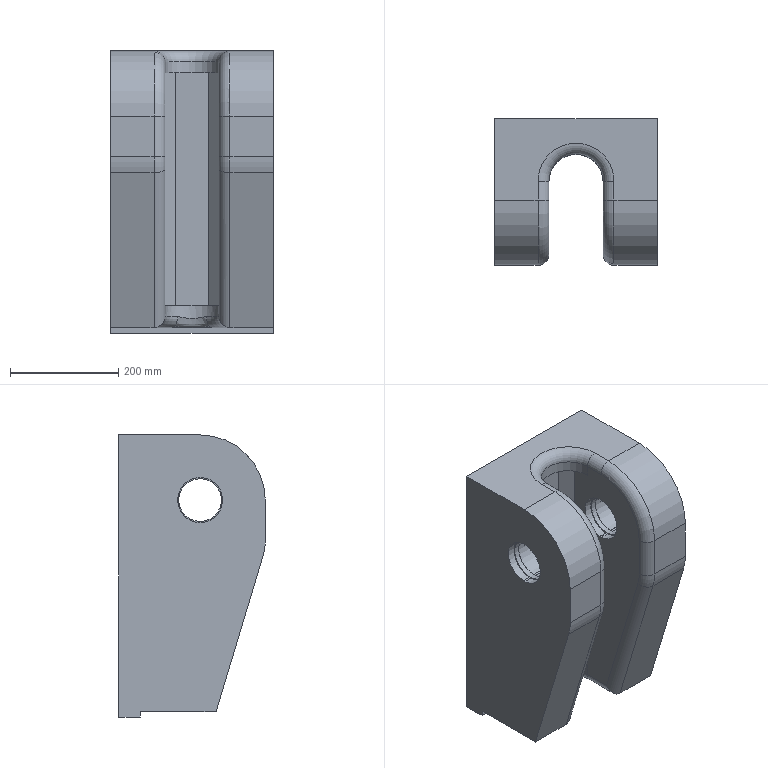Part | NX | features solid 2 | 1 solid | 96 faces | box 300 x 270 x 520 mm | volume 26476228 mm3 | plane 58 | cylinder 30 | torus 7 | spline 1 | commonest cylinder face diameters 83 x12 40 x8 79 x4 100 x2 200 x2 240 x2